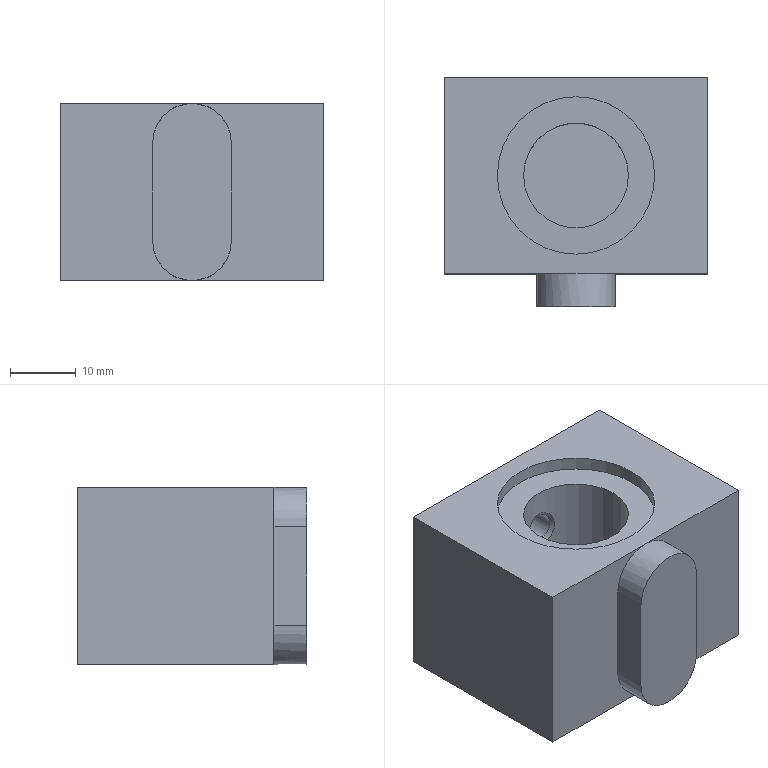Part | NX | features DATUM_CSYS 6, SKETCH 5, EXTRUDE 4, BLEND 1, HOLE PACKAGE 1, SIMPLE HOLE 1, SYMBOLIC_THREAD 1 | 1 solid | 19 faces | box 40 x 35 x 27 mm | volume 30203 mm3 | plane 12 | cylinder 5 | cone 1 | spline 1 | commonest cylinder face diameters 12 x2 5 x1 16 x1 24 x1
STEP:
#1=CARTESIAN_POINT('',(-6.,-15.,-6.));
#2=VERTEX_POINT('',#1);
#3=CARTESIAN_POINT('',(-6.,-15.,-21.));
#4=VERTEX_POINT('',#3);
#5=CARTESIAN_POINT('',(-6.,-15.,-27.));
#6=DIRECTION('',(0.,0.,-1.));
#7=VECTOR('',#6,1000.);
#8=LINE('',#5,#7);
#9=EDGE_CURVE('',#2,#4,#8,.T.);
#10=ORIENTED_EDGE('',*,*,#9,.F.);
#11=CARTESIAN_POINT('',(0.,-15.,0.));
#12=VERTEX_POINT('',#11);
#13=CARTESIAN_POINT('',(0.,-15.,-6.));
#14=DIRECTION('',(0.,-1.,0.));
#15=DIRECTION('',(0.,0.,-1.));
#16=AXIS2_PLACEMENT_3D('',#13,#14,#15);
#17=CIRCLE('',#16,6.);
#18=EDGE_CURVE('',#2,#12,#17,.F.);
#19=ORIENTED_EDGE('',*,*,#18,.T.);
#20=CARTESIAN_POINT('',(-20.,-15.,0.));
#21=VERTEX_POINT('',#20);
#22=CARTESIAN_POINT('',(-20.,-15.,0.));
#23=DIRECTION('',(1.,0.,0.));
#24=VECTOR('',#23,1000.);
#25=LINE('',#22,#24);
#26=EDGE_CURVE('',#21,#12,#25,.T.);
#27=ORIENTED_EDGE('',*,*,#26,.F.);
#28=CARTESIAN_POINT('',(-20.,-15.,-27.));
#29=VERTEX_POINT('',#28);
#30=CARTESIAN_POINT('',(-20.,-15.,-27.));
#31=DIRECTION('',(0.,0.,1.));
#32=VECTOR('',#31,1000.);
#33=LINE('',#30,#32);
#34=EDGE_CURVE('',#29,#21,#33,.T.);
#35=ORIENTED_EDGE('',*,*,#34,.F.);
#36=CARTESIAN_POINT('',(0.,-15.,-27.));
#37=VERTEX_POINT('',#36);
#38=CARTESIAN_POINT('',(-20.,-15.,-27.));
#39=DIRECTION('',(1.,0.,0.));
#40=VECTOR('',#39,1000.);
#41=LINE('',#38,#40);
#42=EDGE_CURVE('',#29,#37,#41,.T.);
#43=ORIENTED_EDGE('',*,*,#42,.T.);
#44=CARTESIAN_POINT('',(0.,-15.,-21.));
#45=DIRECTION('',(0.,-1.,0.));
#46=DIRECTION('',(0.,0.,-1.));
#47=AXIS2_PLACEMENT_3D('',#44,#45,#46);
#48=CIRCLE('',#47,6.);
#49=EDGE_CURVE('',#37,#4,#48,.F.);
#50=ORIENTED_EDGE('',*,*,#49,.T.);
#51=EDGE_LOOP('',(#10,#19,#27,#35,#43,#50));
#52=FACE_BOUND('',#51,.T.);
#53=CARTESIAN_POINT('',(-20.,-15.,-27.));
#54=DIRECTION('',(0.,-1.,0.));
#55=DIRECTION('',(0.,0.,-1.));
#56=AXIS2_PLACEMENT_3D('',#53,#54,#55);
#57=PLANE('',#56);
#58=ADVANCED_FACE('',(#52),#57,.T.);
#59=CARTESIAN_POINT('',(-20.,15.,0.));
#60=VERTEX_POINT('',#59);
#61=CARTESIAN_POINT('',(-20.,15.,0.));
#62=DIRECTION('',(0.,-1.,0.));
#63=VECTOR('',#62,1000.);
#64=LINE('',#61,#63);
#65=EDGE_CURVE('',#60,#21,#64,.T.);
#66=ORIENTED_EDGE('',*,*,#65,.F.);
#67=CARTESIAN_POINT('',(-20.,15.,-27.));
#68=VERTEX_POINT('',#67);
#69=CARTESIAN_POINT('',(-20.,15.,-27.));
#70=DIRECTION('',(0.,0.,1.));
#71=VECTOR('',#70,1000.);
#72=LINE('',#69,#71);
#73=EDGE_CURVE('',#68,#60,#72,.T.);
#74=ORIENTED_EDGE('',*,*,#73,.F.);
#75=CARTESIAN_POINT('',(-20.,15.,-27.));
#76=DIRECTION('',(0.,-1.,0.));
#77=VECTOR('',#76,1000.);
#78=LINE('',#75,#77);
#79=EDGE_CURVE('',#68,#29,#78,.T.);
#80=ORIENTED_EDGE('',*,*,#79,.T.);
#81=ORIENTED_EDGE('',*,*,#34,.T.);
#82=EDGE_LOOP('',(#66,#74,#80,#81));
#83=FACE_BOUND('',#82,.T.);
#84=CARTESIAN_POINT('',(-20.,15.,-27.));
#85=DIRECTION('',(-1.,0.,0.));
#86=DIRECTION('',(0.,0.,1.));
#87=AXIS2_PLACEMENT_3D('',#84,#85,#86);
#88=PLANE('',#87);
#89=ADVANCED_FACE('',(#83),#88,.T.);
#90=CARTESIAN_POINT('',(6.,-15.,-21.));
#91=VERTEX_POINT('',#90);
#92=CARTESIAN_POINT('',(6.,-15.,-6.));
#93=VERTEX_POINT('',#92);
#94=CARTESIAN_POINT('',(6.,-15.,-27.));
#95=DIRECTION('',(0.,0.,1.));
#96=VECTOR('',#95,1000.);
#97=LINE('',#94,#96);
#98=EDGE_CURVE('',#91,#93,#97,.T.);
#99=ORIENTED_EDGE('',*,*,#98,.F.);
#100=CARTESIAN_POINT('',(0.,-15.,-21.));
#101=DIRECTION('',(0.,-1.,0.));
#102=DIRECTION('',(0.,0.,-1.));
#103=AXIS2_PLACEMENT_3D('',#100,#101,#102);
#104=CIRCLE('',#103,6.);
#105=EDGE_CURVE('',#91,#37,#104,.F.);
#106=ORIENTED_EDGE('',*,*,#105,.T.);
#107=CARTESIAN_POINT('',(20.,-15.,-27.));
#108=VERTEX_POINT('',#107);
#109=CARTESIAN_POINT('',(-20.,-15.,-27.));
#110=DIRECTION('',(1.,0.,0.));
#111=VECTOR('',#110,1000.);
#112=LINE('',#109,#111);
#113=EDGE_CURVE('',#37,#108,#112,.T.);
#114=ORIENTED_EDGE('',*,*,#113,.T.);
#115=CARTESIAN_POINT('',(20.,-15.,0.));
#116=VERTEX_POINT('',#115);
#117=CARTESIAN_POINT('',(20.,-15.,-27.));
#118=DIRECTION('',(0.,0.,1.));
#119=VECTOR('',#118,1000.);
#120=LINE('',#117,#119);
#121=EDGE_CURVE('',#108,#116,#120,.T.);
#122=ORIENTED_EDGE('',*,*,#121,.T.);
#123=CARTESIAN_POINT('',(-20.,-15.,0.));
#124=DIRECTION('',(1.,0.,0.));
#125=VECTOR('',#124,1000.);
#126=LINE('',#123,#125);
#127=EDGE_CURVE('',#12,#116,#126,.T.);
#128=ORIENTED_EDGE('',*,*,#127,.F.);
#129=CARTESIAN_POINT('',(0.,-15.,-6.));
#130=DIRECTION('',(0.,-1.,0.));
#131=DIRECTION('',(0.,0.,-1.));
#132=AXIS2_PLACEMENT_3D('',#129,#130,#131);
#133=CIRCLE('',#132,6.);
#134=EDGE_CURVE('',#12,#93,#133,.F.);
#135=ORIENTED_EDGE('',*,*,#134,.T.);
#136=EDGE_LOOP('',(#99,#106,#114,#122,#128,#135));
#137=FACE_BOUND('',#136,.T.);
#138=CARTESIAN_POINT('',(-20.,-15.,-27.));
#139=DIRECTION('',(0.,-1.,0.));
#140=DIRECTION('',(0.,0.,-1.));
#141=AXIS2_PLACEMENT_3D('',#138,#139,#140);
#142=PLANE('',#141);
#143=ADVANCED_FACE('',(#137),#142,.T.);
#144=CARTESIAN_POINT('',(20.,15.,0.));
#145=VERTEX_POINT('',#144);
#146=CARTESIAN_POINT('',(20.,-15.,0.));
#147=DIRECTION('',(0.,1.,0.));
#148=VECTOR('',#147,1000.);
#149=LINE('',#146,#148);
#150=EDGE_CURVE('',#116,#145,#149,.T.);
#151=ORIENTED_EDGE('',*,*,#150,.F.);
#152=ORIENTED_EDGE('',*,*,#121,.F.);
#153=CARTESIAN_POINT('',(20.,15.,-27.));
#154=VERTEX_POINT('',#153);
#155=CARTESIAN_POINT('',(20.,-15.,-27.));
#156=DIRECTION('',(0.,1.,0.));
#157=VECTOR('',#156,1000.);
#158=LINE('',#155,#157);
#159=EDGE_CURVE('',#108,#154,#158,.T.);
#160=ORIENTED_EDGE('',*,*,#159,.T.);
#161=CARTESIAN_POINT('',(20.,15.,-27.));
#162=DIRECTION('',(0.,0.,1.));
#163=VECTOR('',#162,1000.);
#164=LINE('',#161,#163);
#165=EDGE_CURVE('',#154,#145,#164,.T.);
#166=ORIENTED_EDGE('',*,*,#165,.T.);
#167=EDGE_LOOP('',(#151,#152,#160,#166));
#168=FACE_BOUND('',#167,.T.);
#169=CARTESIAN_POINT('',(20.,-15.,-27.));
#170=DIRECTION('',(1.,0.,0.));
#171=DIRECTION('',(0.,0.,-1.));
#172=AXIS2_PLACEMENT_3D('',#169,#170,#171);
#173=PLANE('',#172);
#174=ADVANCED_FACE('',(#168),#173,.T.);
#175=CARTESIAN_POINT('',(0.,15.,-6.));
#176=VERTEX_POINT('',#175);
#177=CARTESIAN_POINT('',(0.,15.,-9.));
#178=DIRECTION('',(0.,1.,0.));
#179=DIRECTION('',(0.,0.,1.));
#180=AXIS2_PLACEMENT_3D('',#177,#178,#179);
#181=CIRCLE('',#180,3.);
#182=EDGE_CURVE('',#176,#176,#181,.F.);
#183=ORIENTED_EDGE('',*,*,#182,.T.);
#184=EDGE_LOOP('',(#183));
#185=FACE_BOUND('',#184,.T.);
#186=CARTESIAN_POINT('',(20.,15.,0.));
#187=DIRECTION('',(-1.,0.,0.));
#188=VECTOR('',#187,1000.);
#189=LINE('',#186,#188);
#190=EDGE_CURVE('',#145,#60,#189,.T.);
#191=ORIENTED_EDGE('',*,*,#190,.F.);
#192=ORIENTED_EDGE('',*,*,#165,.F.);
#193=CARTESIAN_POINT('',(20.,15.,-27.));
#194=DIRECTION('',(-1.,0.,0.));
#195=VECTOR('',#194,1000.);
#196=LINE('',#193,#195);
#197=EDGE_CURVE('',#154,#68,#196,.T.);
#198=ORIENTED_EDGE('',*,*,#197,.T.);
#199=ORIENTED_EDGE('',*,*,#73,.T.);
#200=EDGE_LOOP('',(#191,#192,#198,#199));
#201=FACE_BOUND('',#200,.T.);
#202=CARTESIAN_POINT('',(20.,15.,-27.));
#203=DIRECTION('',(0.,1.,0.));
#204=DIRECTION('',(0.,0.,1.));
#205=AXIS2_PLACEMENT_3D('',#202,#203,#204);
#206=PLANE('',#205);
#207=ADVANCED_FACE('',(#185,#201),#206,.T.);
#208=ORIENTED_EDGE('',*,*,#113,.F.);
#209=ORIENTED_EDGE('',*,*,#42,.F.);
#210=ORIENTED_EDGE('',*,*,#79,.F.);
#211=ORIENTED_EDGE('',*,*,#197,.F.);
#212=ORIENTED_EDGE('',*,*,#159,.F.);
#213=EDGE_LOOP('',(#208,#209,#210,#211,#212));
#214=FACE_BOUND('',#213,.T.);
#215=CARTESIAN_POINT('',(0.,0.,-27.));
#216=DIRECTION('',(0.,0.,1.));
#217=DIRECTION('',(1.,0.,0.));
#218=AXIS2_PLACEMENT_3D('',#215,#216,#217);
#219=PLANE('',#218);
#220=ADVANCED_FACE('',(#214),#219,.F.);
#221=CARTESIAN_POINT('',(12.,0.,0.));
#222=VERTEX_POINT('',#221);
#223=CARTESIAN_POINT('',(0.,0.,0.));
#224=DIRECTION('',(0.,0.,1.));
#225=DIRECTION('',(1.,0.,0.));
#226=AXIS2_PLACEMENT_3D('',#223,#224,#225);
#227=CIRCLE('',#226,12.);
#228=EDGE_CURVE('',#222,#222,#227,.T.);
#229=ORIENTED_EDGE('',*,*,#228,.F.);
#230=EDGE_LOOP('',(#229));
#231=FACE_BOUND('',#230,.T.);
#232=ORIENTED_EDGE('',*,*,#26,.T.);
#233=ORIENTED_EDGE('',*,*,#127,.T.);
#234=ORIENTED_EDGE('',*,*,#150,.T.);
#235=ORIENTED_EDGE('',*,*,#190,.T.);
#236=ORIENTED_EDGE('',*,*,#65,.T.);
#237=EDGE_LOOP('',(#232,#233,#234,#235,#236));
#238=FACE_BOUND('',#237,.T.);
#239=CARTESIAN_POINT('',(0.,0.,0.));
#240=DIRECTION('',(0.,0.,1.));
#241=DIRECTION('',(1.,0.,0.));
#242=AXIS2_PLACEMENT_3D('',#239,#240,#241);
#243=PLANE('',#242);
#244=ADVANCED_FACE('',(#231,#238),#243,.T.);
#245=ORIENTED_EDGE('',*,*,#9,.T.);
#246=CARTESIAN_POINT('',(-6.,-20.,-21.));
#247=VERTEX_POINT('',#246);
#248=CARTESIAN_POINT('',(-6.,-20.,-21.));
#249=DIRECTION('',(0.,1.,0.));
#250=VECTOR('',#249,1000.);
#251=LINE('',#248,#250);
#252=EDGE_CURVE('',#4,#247,#251,.F.);
#253=ORIENTED_EDGE('',*,*,#252,.T.);
#254=CARTESIAN_POINT('',(-6.,-20.,-6.));
#255=VERTEX_POINT('',#254);
#256=CARTESIAN_POINT('',(-6.,-20.,-27.));
#257=DIRECTION('',(0.,0.,1.));
#258=VECTOR('',#257,1000.);
#259=LINE('',#256,#258);
#260=EDGE_CURVE('',#247,#255,#259,.T.);
#261=ORIENTED_EDGE('',*,*,#260,.T.);
#262=CARTESIAN_POINT('',(-6.,-10.,-6.));
#263=DIRECTION('',(0.,1.,0.));
#264=VECTOR('',#263,1000.);
#265=LINE('',#262,#264);
#266=EDGE_CURVE('',#255,#2,#265,.T.);
#267=ORIENTED_EDGE('',*,*,#266,.T.);
#268=EDGE_LOOP('',(#245,#253,#261,#267));
#269=FACE_BOUND('',#268,.T.);
#270=CARTESIAN_POINT('',(-6.,-10.,-27.));
#271=DIRECTION('',(-1.,0.,0.));
#272=DIRECTION('',(0.,-1.,0.));
#273=AXIS2_PLACEMENT_3D('',#270,#271,#272);
#274=PLANE('',#273);
#275=ADVANCED_FACE('',(#269),#274,.T.);
#276=ORIENTED_EDGE('',*,*,#260,.F.);
#277=CARTESIAN_POINT('',(6.,-20.,-21.));
#278=VERTEX_POINT('',#277);
#279=CARTESIAN_POINT('',(0.,-20.,-21.));
#280=DIRECTION('',(0.,-1.,0.));
#281=DIRECTION('',(0.,0.,-1.));
#282=AXIS2_PLACEMENT_3D('',#279,#280,#281);
#283=CIRCLE('',#282,6.);
#284=EDGE_CURVE('',#247,#278,#283,.T.);
#285=ORIENTED_EDGE('',*,*,#284,.T.);
#286=CARTESIAN_POINT('',(6.,-20.,-6.));
#287=VERTEX_POINT('',#286);
#288=CARTESIAN_POINT('',(6.,-20.,-27.));
#289=DIRECTION('',(0.,0.,1.));
#290=VECTOR('',#289,1000.);
#291=LINE('',#288,#290);
#292=EDGE_CURVE('',#278,#287,#291,.T.);
#293=ORIENTED_EDGE('',*,*,#292,.T.);
#294=CARTESIAN_POINT('',(0.,-20.,-6.));
#295=DIRECTION('',(0.,-1.,0.));
#296=DIRECTION('',(0.,0.,-1.));
#297=AXIS2_PLACEMENT_3D('',#294,#295,#296);
#298=CIRCLE('',#297,6.);
#299=EDGE_CURVE('',#287,#255,#298,.T.);
#300=ORIENTED_EDGE('',*,*,#299,.T.);
#301=EDGE_LOOP('',(#276,#285,#293,#300));
#302=FACE_BOUND('',#301,.T.);
#303=CARTESIAN_POINT('',(-6.,-20.,-27.));
#304=DIRECTION('',(0.,-1.,0.));
#305=DIRECTION('',(0.,0.,-1.));
#306=AXIS2_PLACEMENT_3D('',#303,#304,#305);
#307=PLANE('',#306);
#308=ADVANCED_FACE('',(#302),#307,.T.);
#309=ORIENTED_EDGE('',*,*,#292,.F.);
#310=CARTESIAN_POINT('',(6.,-15.,-21.));
#311=DIRECTION('',(0.,-1.,0.));
#312=VECTOR('',#311,1000.);
#313=LINE('',#310,#312);
#314=EDGE_CURVE('',#278,#91,#313,.F.);
#315=ORIENTED_EDGE('',*,*,#314,.T.);
#316=ORIENTED_EDGE('',*,*,#98,.T.);
#317=CARTESIAN_POINT('',(6.,-20.,-6.));
#318=DIRECTION('',(0.,-1.,0.));
#319=VECTOR('',#318,1000.);
#320=LINE('',#317,#319);
#321=EDGE_CURVE('',#93,#287,#320,.T.);
#322=ORIENTED_EDGE('',*,*,#321,.T.);
#323=EDGE_LOOP('',(#309,#315,#316,#322));
#324=FACE_BOUND('',#323,.T.);
#325=CARTESIAN_POINT('',(6.,-20.,-27.));
#326=DIRECTION('',(1.,0.,0.));
#327=DIRECTION('',(0.,0.,-1.));
#328=AXIS2_PLACEMENT_3D('',#325,#326,#327);
#329=PLANE('',#328);
#330=ADVANCED_FACE('',(#324),#329,.T.);
#331=ORIENTED_EDGE('',*,*,#314,.F.);
#332=ORIENTED_EDGE('',*,*,#284,.F.);
#333=ORIENTED_EDGE('',*,*,#252,.F.);
#334=ORIENTED_EDGE('',*,*,#49,.F.);
#335=ORIENTED_EDGE('',*,*,#105,.F.);
#336=EDGE_LOOP('',(#331,#332,#333,#334,#335));
#337=FACE_BOUND('',#336,.T.);
#338=CARTESIAN_POINT('',(0.,0.,-21.));
#339=DIRECTION('',(0.,1.,0.));
#340=DIRECTION('',(0.,0.,1.));
#341=AXIS2_PLACEMENT_3D('',#338,#339,#340);
#342=CYLINDRICAL_SURFACE('',#341,6.);
#343=ADVANCED_FACE('',(#337),#342,.T.);
#344=ORIENTED_EDGE('',*,*,#134,.F.);
#345=ORIENTED_EDGE('',*,*,#18,.F.);
#346=ORIENTED_EDGE('',*,*,#266,.F.);
#347=ORIENTED_EDGE('',*,*,#299,.F.);
#348=ORIENTED_EDGE('',*,*,#321,.F.);
#349=EDGE_LOOP('',(#344,#345,#346,#347,#348));
#350=FACE_BOUND('',#349,.T.);
#351=CARTESIAN_POINT('',(0.,-20.,-6.));
#352=DIRECTION('',(0.,-1.,0.));
#353=DIRECTION('',(0.,0.,-1.));
#354=AXIS2_PLACEMENT_3D('',#351,#352,#353);
#355=CYLINDRICAL_SURFACE('',#354,6.);
#356=ADVANCED_FACE('',(#350),#355,.T.);
#357=CARTESIAN_POINT('',(12.,0.,-2.));
#358=VERTEX_POINT('',#357);
#359=CARTESIAN_POINT('',(0.,0.,-2.));
#360=DIRECTION('',(0.,0.,1.));
#361=DIRECTION('',(1.,0.,0.));
#362=AXIS2_PLACEMENT_3D('',#359,#360,#361);
#363=CIRCLE('',#362,12.);
#364=EDGE_CURVE('',#358,#358,#363,.F.);
#365=ORIENTED_EDGE('',*,*,#364,.T.);
#366=EDGE_LOOP('',(#365));
#367=FACE_BOUND('',#366,.T.);
#368=ORIENTED_EDGE('',*,*,#228,.T.);
#369=EDGE_LOOP('',(#368));
#370=FACE_BOUND('',#369,.T.);
#371=CARTESIAN_POINT('',(0.,0.,-2.));
#372=DIRECTION('',(0.,0.,1.));
#373=DIRECTION('',(1.,0.,0.));
#374=AXIS2_PLACEMENT_3D('',#371,#372,#373);
#375=CYLINDRICAL_SURFACE('',#374,12.);
#376=ADVANCED_FACE('',(#367,#370),#375,.F.);
#377=CARTESIAN_POINT('',(8.,0.,-2.));
#378=VERTEX_POINT('',#377);
#379=CARTESIAN_POINT('',(0.,0.,-2.));
#380=DIRECTION('',(0.,0.,1.));
#381=DIRECTION('',(1.,0.,0.));
#382=AXIS2_PLACEMENT_3D('',#379,#380,#381);
#383=CIRCLE('',#382,8.);
#384=EDGE_CURVE('',#378,#378,#383,.T.);
#385=ORIENTED_EDGE('',*,*,#384,.F.);
#386=EDGE_LOOP('',(#385));
#387=FACE_BOUND('',#386,.T.);
#388=ORIENTED_EDGE('',*,*,#364,.F.);
#389=EDGE_LOOP('',(#388));
#390=FACE_BOUND('',#389,.T.);
#391=CARTESIAN_POINT('',(0.,0.,-2.));
#392=DIRECTION('',(0.,0.,1.));
#393=DIRECTION('',(1.,0.,0.));
#394=AXIS2_PLACEMENT_3D('',#391,#392,#393);
#395=PLANE('',#394);
#396=ADVANCED_FACE('',(#387,#390),#395,.T.);
#397=CARTESIAN_POINT('',(0.,8.,-12.102));
#398=VERTEX_POINT('',#397);
#399=CARTESIAN_POINT('',(1.169,7.939,-11.917));
#400=CARTESIAN_POINT('',(0.03784,8.028,-12.187));
#401=CARTESIAN_POINT('',(-1.088,7.949,-11.946));
#402=CARTESIAN_POINT('',(-2.032,7.753,-11.294));
#403=CARTESIAN_POINT('',(-2.675,7.544,-10.288));
#404=CARTESIAN_POINT('',(-2.934,7.442,-9.067));
#405=CARTESIAN_POINT('',(-2.724,7.526,-7.841));
#406=CARTESIAN_POINT('',(-2.114,7.73,-6.794));
#407=CARTESIAN_POINT('',(-1.186,7.935,-6.094));
#408=CARTESIAN_POINT('',(-0.06312,8.028,-5.814));
#409=CARTESIAN_POINT('',(1.068,7.953,-6.04));
#410=CARTESIAN_POINT('',(2.03,7.753,-6.704));
#411=CARTESIAN_POINT('',(2.674,7.544,-7.713));
#412=CARTESIAN_POINT('',(2.933,7.442,-8.935));
#413=CARTESIAN_POINT('',(2.724,7.526,-10.16));
#414=CARTESIAN_POINT('',(2.115,7.729,-11.205));
#415=CARTESIAN_POINT('',(1.169,7.939,-11.917));
#416=CARTESIAN_POINT('',(0.03784,8.028,-12.187));
#417=CARTESIAN_POINT('',(-1.088,7.949,-11.946));
#418=B_SPLINE_CURVE_WITH_KNOTS('',3,(#399,#400,#401,#402,#403,#404,#405,#406,#407,#408,#409,#410,#411,#412,#413,#414,#415,#416,#417),.UNSPECIFIED.,.T.,.F.,(1,1,1,1,1,1,1,1,1,1,1,1,1,1,1,1,1,1,1,1,1,1,1),(-0.1908,-0.1283,-0.06579,0.,0.05937,0.1217,0.1842,0.2467,0.3092,0.3717,0.4342,0.4967,0.5592,0.6217,0.6842,0.7467,0.8092,0.8717,0.9342,1.,1.059,1.122,1.184),.UNSPECIFIED.);
#419=EDGE_CURVE('',#398,#398,#418,.T.);
#420=ORIENTED_EDGE('',*,*,#419,.T.);
#421=EDGE_LOOP('',(#420));
#422=FACE_BOUND('',#421,.T.);
#423=ORIENTED_EDGE('',*,*,#384,.T.);
#424=EDGE_LOOP('',(#423));
#425=FACE_BOUND('',#424,.T.);
#426=CARTESIAN_POINT('',(8.,0.,-15.));
#427=VERTEX_POINT('',#426);
#428=CARTESIAN_POINT('',(0.,0.,-15.));
#429=DIRECTION('',(0.,0.,1.));
#430=DIRECTION('',(1.,0.,0.));
#431=AXIS2_PLACEMENT_3D('',#428,#429,#430);
#432=CIRCLE('',#431,8.);
#433=EDGE_CURVE('',#427,#427,#432,.F.);
#434=ORIENTED_EDGE('',*,*,#433,.T.);
#435=EDGE_LOOP('',(#434));
#436=FACE_BOUND('',#435,.T.);
#437=CARTESIAN_POINT('',(0.,0.,-15.));
#438=DIRECTION('',(0.,0.,1.));
#439=DIRECTION('',(1.,0.,0.));
#440=AXIS2_PLACEMENT_3D('',#437,#438,#439);
#441=CYLINDRICAL_SURFACE('',#440,8.);
#442=ADVANCED_FACE('',(#422,#425,#436),#441,.F.);
#443=ORIENTED_EDGE('',*,*,#433,.F.);
#444=EDGE_LOOP('',(#443));
#445=FACE_BOUND('',#444,.T.);
#446=CARTESIAN_POINT('',(0.,0.,-15.));
#447=DIRECTION('',(0.,0.,1.));
#448=DIRECTION('',(1.,0.,0.));
#449=AXIS2_PLACEMENT_3D('',#446,#447,#448);
#450=PLANE('',#449);
#451=ADVANCED_FACE('',(#445),#450,.T.);
#452=CARTESIAN_POINT('',(0.,8.69,-11.5));
#453=VERTEX_POINT('',#452);
#454=CARTESIAN_POINT('',(-0.8632,8.646,-11.427));
#455=CARTESIAN_POINT('',(-0.02704,8.71,-11.535));
#456=CARTESIAN_POINT('',(0.7755,8.651,-11.434));
#457=CARTESIAN_POINT('',(1.748,8.441,-10.922));
#458=CARTESIAN_POINT('',(2.417,8.172,-9.889));
#459=CARTESIAN_POINT('',(2.527,8.097,-9.061));
#460=CARTESIAN_POINT('',(2.468,8.146,-8.316));
#461=CARTESIAN_POINT('',(1.939,8.372,-7.261));
#462=CARTESIAN_POINT('',(0.9196,8.635,-6.598));
#463=CARTESIAN_POINT('',(0.0674,8.709,-6.466));
#464=CARTESIAN_POINT('',(-0.7169,8.661,-6.545));
#465=CARTESIAN_POINT('',(-1.731,8.447,-7.055));
#466=CARTESIAN_POINT('',(-2.417,8.173,-8.108));
#467=CARTESIAN_POINT('',(-2.527,8.097,-8.94));
#468=CARTESIAN_POINT('',(-2.467,8.145,-9.683));
#469=CARTESIAN_POINT('',(-1.93,8.377,-10.758));
#470=CARTESIAN_POINT('',(-0.8632,8.646,-11.427));
#471=CARTESIAN_POINT('',(-0.02704,8.71,-11.535));
#472=CARTESIAN_POINT('',(0.7755,8.651,-11.434));
#473=B_SPLINE_CURVE_WITH_KNOTS('',3,(#454,#455,#456,#457,#458,#459,#460,#461,#462,#463,#464,#465,#466,#467,#468,#469,#470,#471,#472),.UNSPECIFIED.,.T.,.F.,(1,1,1,1,1,1,1,1,1,1,1,1,1,1,1,1,1,1,1,1,1,1,1),(-0.1941,-0.1316,-0.06579,0.,0.05937,0.1187,0.1811,0.2434,0.3059,0.3684,0.4309,0.4934,0.5559,0.6184,0.6809,0.7434,0.8059,0.8684,0.9342,1.,1.059,1.119,1.181),.UNSPECIFIED.);
#474=EDGE_CURVE('',#453,#453,#473,.T.);
#475=ORIENTED_EDGE('',*,*,#474,.T.);
#476=EDGE_LOOP('',(#475));
#477=FACE_BOUND('',#476,.T.);
#478=CARTESIAN_POINT('',(0.,14.5,-6.5));
#479=VERTEX_POINT('',#478);
#480=CARTESIAN_POINT('',(0.,14.5,-9.));
#481=DIRECTION('',(0.,1.,0.));
#482=DIRECTION('',(0.,0.,1.));
#483=AXIS2_PLACEMENT_3D('',#480,#481,#482);
#484=CIRCLE('',#483,2.5);
#485=EDGE_CURVE('',#479,#479,#484,.T.);
#486=ORIENTED_EDGE('',*,*,#485,.T.);
#487=EDGE_LOOP('',(#486));
#488=FACE_BOUND('',#487,.T.);
#489=CARTESIAN_POINT('',(0.,15.,-9.));
#490=DIRECTION('',(0.,-1.,0.));
#491=DIRECTION('',(0.,0.,-1.));
#492=AXIS2_PLACEMENT_3D('',#489,#490,#491);
#493=CYLINDRICAL_SURFACE('',#492,2.5);
#494=ADVANCED_FACE('',(#477,#488),#493,.F.);
#495=ORIENTED_EDGE('',*,*,#485,.F.);
#496=EDGE_LOOP('',(#495));
#497=FACE_BOUND('',#496,.T.);
#498=ORIENTED_EDGE('',*,*,#182,.F.);
#499=EDGE_LOOP('',(#498));
#500=FACE_BOUND('',#499,.T.);
#501=CARTESIAN_POINT('',(0.,15.,-9.));
#502=DIRECTION('',(0.,1.,0.));
#503=DIRECTION('',(0.,0.,1.));
#504=AXIS2_PLACEMENT_3D('',#501,#502,#503);
#505=CONICAL_SURFACE('',#504,3.,0.7854);
#506=ADVANCED_FACE('',(#497,#500),#505,.F.);
#507=ORIENTED_EDGE('',*,*,#474,.F.);
#508=EDGE_LOOP('',(#507));
#509=FACE_BOUND('',#508,.T.);
#510=ORIENTED_EDGE('',*,*,#419,.F.);
#511=EDGE_LOOP('',(#510));
#512=FACE_BOUND('',#511,.T.);
#513=CARTESIAN_POINT('',(0.7568,8.,-12.102));
#514=CARTESIAN_POINT('',(-0.7568,8.,-12.103));
#515=CARTESIAN_POINT('',(-1.497,7.88,-11.762));
#516=CARTESIAN_POINT('',(-2.544,7.602,-10.624));
#517=CARTESIAN_POINT('',(-2.856,7.473,-9.825));
#518=CARTESIAN_POINT('',(-2.856,7.473,-8.18));
#519=CARTESIAN_POINT('',(-2.544,7.602,-7.376));
#520=CARTESIAN_POINT('',(-1.495,7.88,-6.236));
#521=CARTESIAN_POINT('',(-0.7597,8.,-5.899));
#522=CARTESIAN_POINT('',(0.755,8.,-5.897));
#523=CARTESIAN_POINT('',(1.495,7.88,-6.236));
#524=CARTESIAN_POINT('',(2.543,7.602,-7.376));
#525=CARTESIAN_POINT('',(2.855,7.473,-8.177));
#526=CARTESIAN_POINT('',(2.857,7.472,-9.822));
#527=CARTESIAN_POINT('',(2.544,7.602,-10.624));
#528=CARTESIAN_POINT('',(1.496,7.88,-11.762));
#529=CARTESIAN_POINT('',(0.7568,8.,-12.102));
#530=CARTESIAN_POINT('',(-0.7568,8.,-12.103));
#531=CARTESIAN_POINT('',(0.6624,8.689,-11.5));
#532=CARTESIAN_POINT('',(-0.6624,8.69,-11.5));
#533=CARTESIAN_POINT('',(-1.31,8.559,-11.226));
#534=CARTESIAN_POINT('',(-2.227,8.257,-10.309));
#535=CARTESIAN_POINT('',(-2.5,8.117,-9.664));
#536=CARTESIAN_POINT('',(-2.5,8.117,-8.339));
#537=CARTESIAN_POINT('',(-2.227,8.257,-7.691));
#538=CARTESIAN_POINT('',(-1.308,8.559,-6.773));
#539=CARTESIAN_POINT('',(-0.665,8.689,-6.501));
#540=CARTESIAN_POINT('',(0.6609,8.69,-6.499));
#541=CARTESIAN_POINT('',(1.309,8.559,-6.773));
#542=CARTESIAN_POINT('',(2.226,8.257,-7.691));
#543=CARTESIAN_POINT('',(2.499,8.117,-8.337));
#544=CARTESIAN_POINT('',(2.501,8.117,-9.662));
#545=CARTESIAN_POINT('',(2.227,8.257,-10.309));
#546=CARTESIAN_POINT('',(1.309,8.559,-11.226));
#547=CARTESIAN_POINT('',(0.6624,8.689,-11.5));
#548=CARTESIAN_POINT('',(-0.6624,8.69,-11.5));
#549=B_SPLINE_SURFACE_WITH_KNOTS('',1,3,((#513,#514,#515,#516,#517,#518,#519,#520,#521,#522,#523,#524,#525,#526,#527,#528,#529,#530),(#531,#532,#533,#534,#535,#536,#537,#538,#539,#540,#541,#542,#543,#544,#545,#546,#547,#548)),.RULED_SURF.,.F.,.T.,.F.,(2,2),(2,2,2,2,2,2,2,2,2,2,2),(0.,1.),(-0.001355,0.001087,0.003528,0.00597,0.008411,0.01085,0.01329,0.01574,0.01818,0.02062,0.02306),.UNSPECIFIED.);
#550=ADVANCED_FACE('',(#509,#512),#549,.T.);
#551=CLOSED_SHELL('',(#58,#89,#143,#174,#207,#220,#244,#275,#308,#330,#343,#356,#376,#396,#442,#451,#494,#506,#550));
#552=MANIFOLD_SOLID_BREP('',#551);
#553=(LENGTH_UNIT()NAMED_UNIT(*)SI_UNIT(.MILLI.,.METRE.));
#554=UNCERTAINTY_MEASURE_WITH_UNIT(LENGTH_MEASURE(0.0508),#553,'','');
#555=(NAMED_UNIT(*)PLANE_ANGLE_UNIT()SI_UNIT($,.RADIAN.));
#556=(NAMED_UNIT(*)SI_UNIT($,.STERADIAN.)SOLID_ANGLE_UNIT());
#557=(GEOMETRIC_REPRESENTATION_CONTEXT(3)GLOBAL_UNCERTAINTY_ASSIGNED_CONTEXT((#554))GLOBAL_UNIT_ASSIGNED_CONTEXT((#553,#555,#556))REPRESENTATION_CONTEXT('',''));
#558=ADVANCED_BREP_SHAPE_REPRESENTATION('',(#552),#557);